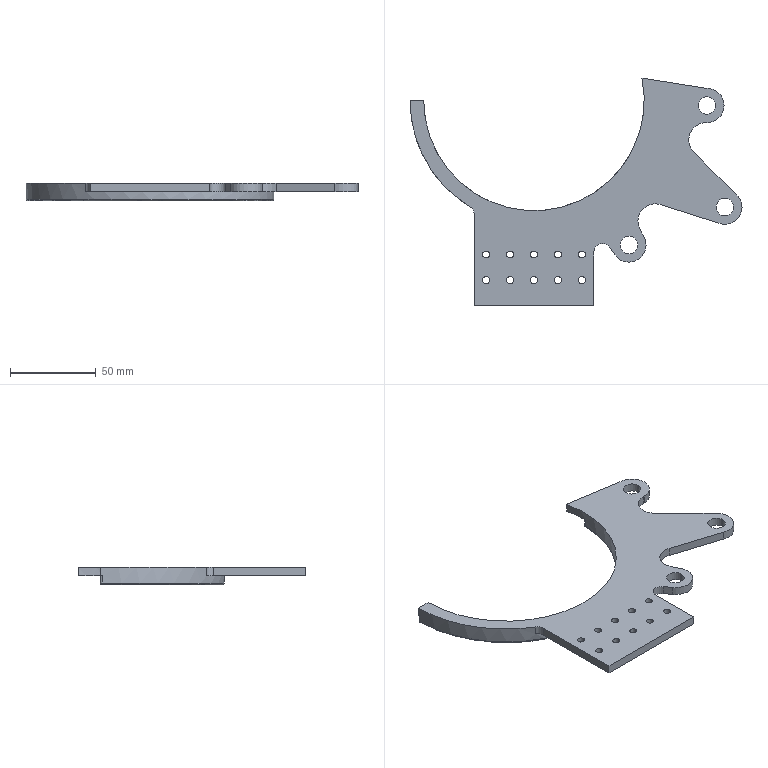Part | STEP file | Half-gear guide groove revised | 1 solid | 68 faces | box 193.874 x 133 x 10.2 mm | volume 53575 mm3 | cylinder 45 | plane 16 | sphere 5 | torus 2 | commonest cylinder face diameters 4.1 x20 20 x8 2 x7 10.2 x6 10 x2 128.8 x1